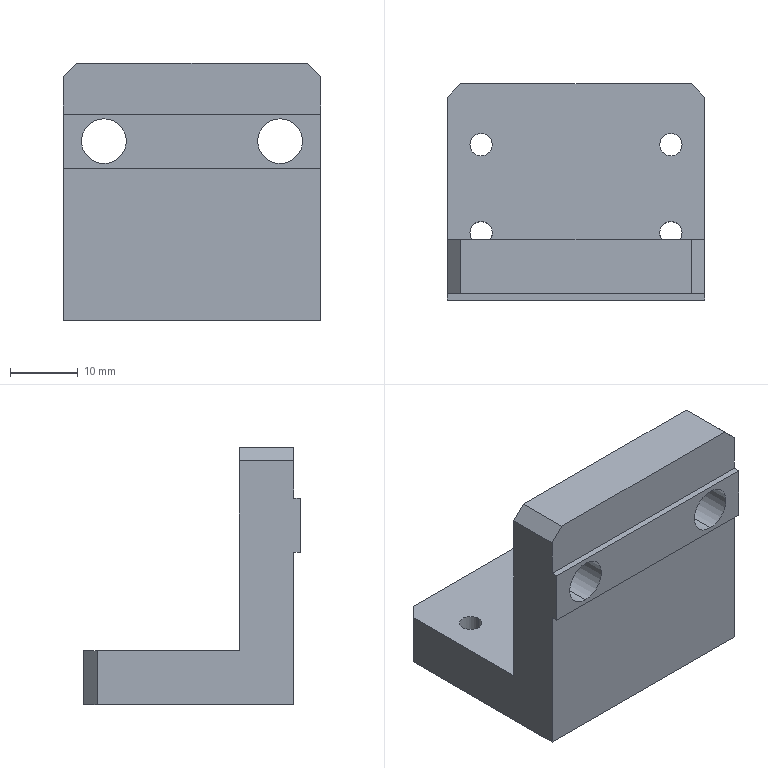Part | STEP file | Cylinder mounting plate | 1 solid | 30 faces | box 38 x 32 x 38 mm | volume 17881 mm3 | plane 16 | cylinder 12 | cone 2 | commonest cylinder face diameters 3.3 x8 6.6 x4